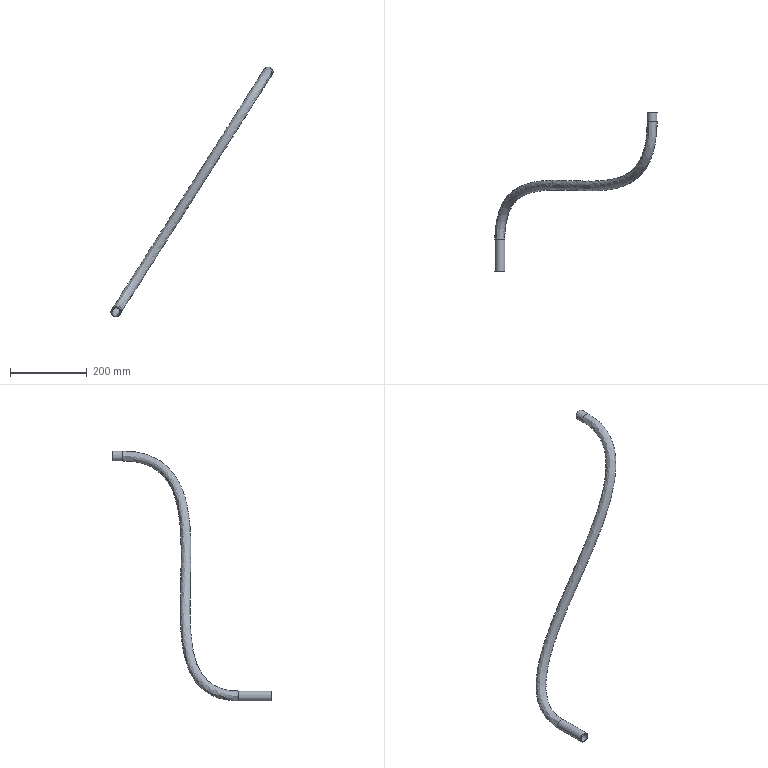Part | STEP file | Part 8^JBJ-F-0000-00 | 1 solid | 8 faces | box 423.697 x 414.992 x 653.065 mm | volume 153249 mm3 | cylinder 4 | spline 2 | plane 2 | commonest cylinder face diameters 22 x2 26 x2